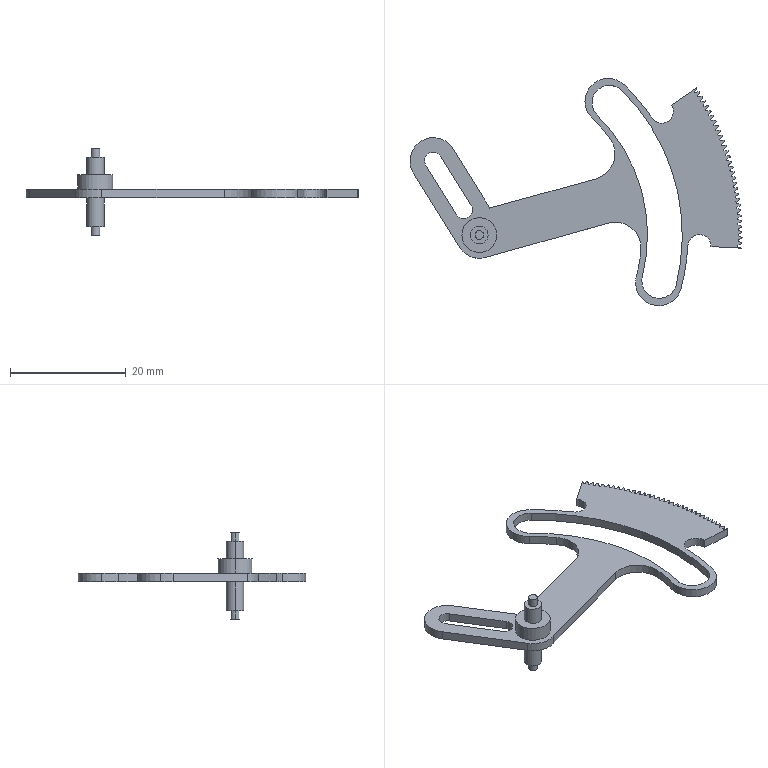Part | SolidWorks | features ICE 6, Extrusion 1 | 1 solid | 172 faces | box 57.266 x 39.218 x 15 mm | volume 1123 mm3 | cylinder 157 | plane 15 | commonest cylinder face diameters 36 x62 89.248 x31 90.6 x30 3 x7 8 x7 6 x6